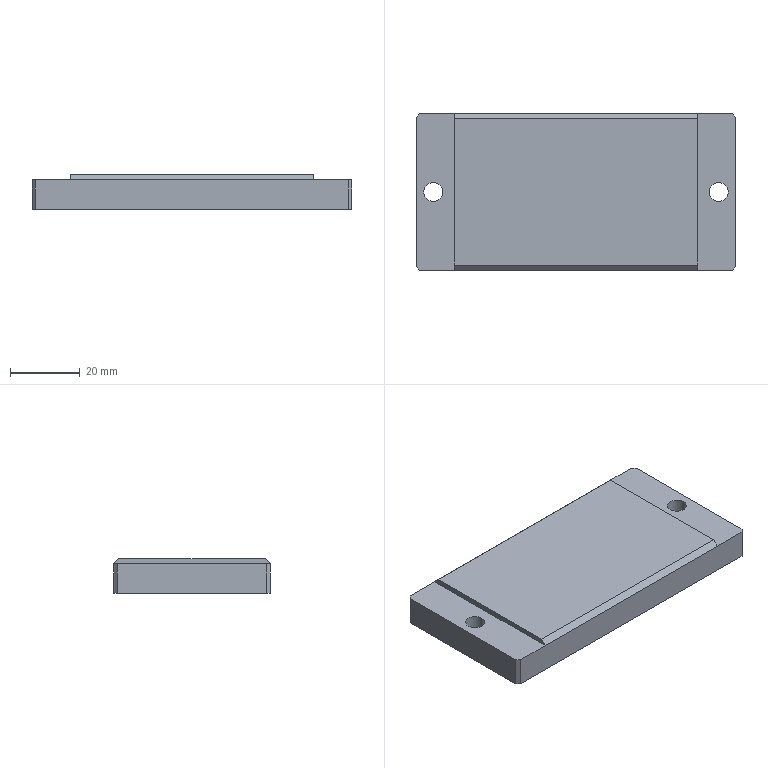Part | STEP file | 2022 Hold-down plate | 1 solid | 20 faces | box 92 x 45 x 10 mm | volume 39337 mm3 | plane 16 | cylinder 4 | commonest cylinder face diameters 5.5 x4
STEP:
#1=CARTESIAN_POINT('',(0.,0.,0.));
#2=DIRECTION('',(0.,0.,1.));
#3=DIRECTION('',(1.,0.,0.));
#4=AXIS2_PLACEMENT_3D('',#1,#2,#3);
#5=CARTESIAN_POINT('',(38.25,0.,8.5));
#6=VERTEX_POINT('',#5);
#7=CARTESIAN_POINT('',(38.25,0.,0.));
#8=VERTEX_POINT('',#7);
#9=CARTESIAN_POINT('',(38.25,0.,10.));
#10=DIRECTION('',(0.,0.,-1.));
#11=VECTOR('',#10,1.);
#12=LINE('',#9,#11);
#13=CARTESIAN_POINT('',(41.,0.,10.));
#14=DIRECTION('',(0.,0.,-1.));
#15=DIRECTION('',(-1.,0.,0.));
#16=AXIS2_PLACEMENT_3D('',#13,#14,#15);
#17=CYLINDRICAL_SURFACE('',#16,2.75);
#18=CARTESIAN_POINT('',(6.283,0.));
#19=DIRECTION('',(0.,1.));
#20=VECTOR('',#19,1.);
#21=LINE('',#18,#20);
#22=(GEOMETRIC_REPRESENTATION_CONTEXT(2)PARAMETRIC_REPRESENTATION_CONTEXT()REPRESENTATION_CONTEXT('',''));
#23=DEFINITIONAL_REPRESENTATION('',(#21),#22);
#24=PCURVE('',#17,#23);
#25=CARTESIAN_POINT('',(41.,0.,10.));
#26=DIRECTION('',(0.,0.,-1.));
#27=DIRECTION('',(-1.,0.,0.));
#28=AXIS2_PLACEMENT_3D('',#25,#26,#27);
#29=CYLINDRICAL_SURFACE('',#28,2.75);
#30=CARTESIAN_POINT('',(0.,0.));
#31=DIRECTION('',(0.,1.));
#32=VECTOR('',#31,1.);
#33=LINE('',#30,#32);
#34=(GEOMETRIC_REPRESENTATION_CONTEXT(2)PARAMETRIC_REPRESENTATION_CONTEXT()REPRESENTATION_CONTEXT('',''));
#35=DEFINITIONAL_REPRESENTATION('',(#33),#34);
#36=PCURVE('',#29,#35);
#37=SURFACE_CURVE('',#12,(#24,#36),.PCURVE_S1.);
#38=EDGE_CURVE('',#6,#8,#37,.T.);
#39=ORIENTED_EDGE('',*,*,#38,.T.);
#40=CARTESIAN_POINT('',(43.75,0.,0.));
#41=VERTEX_POINT('',#40);
#42=CARTESIAN_POINT('',(41.,0.,0.));
#43=DIRECTION('',(0.,0.,-1.));
#44=DIRECTION('',(-1.,0.,0.));
#45=AXIS2_PLACEMENT_3D('',#42,#43,#44);
#46=CIRCLE('',#45,2.75);
#47=CARTESIAN_POINT('',(0.,10.));
#48=DIRECTION('',(1.,0.));
#49=VECTOR('',#48,1.);
#50=LINE('',#47,#49);
#51=(GEOMETRIC_REPRESENTATION_CONTEXT(2)PARAMETRIC_REPRESENTATION_CONTEXT()REPRESENTATION_CONTEXT('',''));
#52=DEFINITIONAL_REPRESENTATION('',(#50),#51);
#53=PCURVE('',#17,#52);
#54=CARTESIAN_POINT('',(0.,0.,0.));
#55=DIRECTION('',(0.,0.,-1.));
#56=DIRECTION('',(-1.,0.,0.));
#57=AXIS2_PLACEMENT_3D('',#54,#55,#56);
#58=PLANE('',#57);
#59=CARTESIAN_POINT('',(-41.,0.));
#60=DIRECTION('',(1.,0.));
#61=AXIS2_PLACEMENT_2D('',#59,#60);
#62=CIRCLE('',#61,2.75);
#63=(GEOMETRIC_REPRESENTATION_CONTEXT(2)PARAMETRIC_REPRESENTATION_CONTEXT()REPRESENTATION_CONTEXT('',''));
#64=DEFINITIONAL_REPRESENTATION('',(#62),#63);
#65=PCURVE('',#58,#64);
#66=SURFACE_CURVE('',#46,(#53,#65),.PCURVE_S1.);
#67=EDGE_CURVE('',#41,#8,#66,.T.);
#68=ORIENTED_EDGE('',*,*,#67,.F.);
#69=CARTESIAN_POINT('',(43.75,0.,8.5));
#70=VERTEX_POINT('',#69);
#71=CARTESIAN_POINT('',(43.75,0.,10.));
#72=DIRECTION('',(0.,0.,-1.));
#73=VECTOR('',#72,1.);
#74=LINE('',#71,#73);
#75=CARTESIAN_POINT('',(3.142,0.));
#76=DIRECTION('',(0.,1.));
#77=VECTOR('',#76,1.);
#78=LINE('',#75,#77);
#79=(GEOMETRIC_REPRESENTATION_CONTEXT(2)PARAMETRIC_REPRESENTATION_CONTEXT()REPRESENTATION_CONTEXT('',''));
#80=DEFINITIONAL_REPRESENTATION('',(#78),#79);
#81=PCURVE('',#17,#80);
#82=CARTESIAN_POINT('',(3.142,0.));
#83=DIRECTION('',(0.,1.));
#84=VECTOR('',#83,1.);
#85=LINE('',#82,#84);
#86=(GEOMETRIC_REPRESENTATION_CONTEXT(2)PARAMETRIC_REPRESENTATION_CONTEXT()REPRESENTATION_CONTEXT('',''));
#87=DEFINITIONAL_REPRESENTATION('',(#85),#86);
#88=PCURVE('',#29,#87);
#89=SURFACE_CURVE('',#74,(#81,#88),.PCURVE_S1.);
#90=EDGE_CURVE('',#70,#41,#89,.T.);
#91=ORIENTED_EDGE('',*,*,#90,.F.);
#92=CARTESIAN_POINT('',(41.,0.,8.5));
#93=DIRECTION('',(0.,0.,-1.));
#94=DIRECTION('',(-1.,0.,0.));
#95=AXIS2_PLACEMENT_3D('',#92,#93,#94);
#96=CIRCLE('',#95,2.75);
#97=CARTESIAN_POINT('',(0.,1.5));
#98=DIRECTION('',(1.,0.));
#99=VECTOR('',#98,1.);
#100=LINE('',#97,#99);
#101=(GEOMETRIC_REPRESENTATION_CONTEXT(2)PARAMETRIC_REPRESENTATION_CONTEXT()REPRESENTATION_CONTEXT('',''));
#102=DEFINITIONAL_REPRESENTATION('',(#100),#101);
#103=PCURVE('',#17,#102);
#104=CARTESIAN_POINT('',(0.,0.,8.5));
#105=DIRECTION('',(0.,0.,-1.));
#106=DIRECTION('',(-1.,0.,0.));
#107=AXIS2_PLACEMENT_3D('',#104,#105,#106);
#108=PLANE('',#107);
#109=CARTESIAN_POINT('',(-41.,0.));
#110=DIRECTION('',(1.,0.));
#111=AXIS2_PLACEMENT_2D('',#109,#110);
#112=CIRCLE('',#111,2.75);
#113=(GEOMETRIC_REPRESENTATION_CONTEXT(2)PARAMETRIC_REPRESENTATION_CONTEXT()REPRESENTATION_CONTEXT('',''));
#114=DEFINITIONAL_REPRESENTATION('',(#112),#113);
#115=PCURVE('',#108,#114);
#116=SURFACE_CURVE('',#96,(#103,#115),.PCURVE_S1.);
#117=EDGE_CURVE('',#70,#6,#116,.T.);
#118=ORIENTED_EDGE('',*,*,#117,.T.);
#119=EDGE_LOOP('',(#39,#68,#91,#118));
#120=FACE_BOUND('',#119,.F.);
#121=ADVANCED_FACE('',(#120),#17,.F.);
#122=CARTESIAN_POINT('',(-43.75,0.,8.5));
#123=VERTEX_POINT('',#122);
#124=CARTESIAN_POINT('',(-43.75,0.,0.));
#125=VERTEX_POINT('',#124);
#126=CARTESIAN_POINT('',(-43.75,0.,10.));
#127=DIRECTION('',(0.,0.,-1.));
#128=VECTOR('',#127,1.);
#129=LINE('',#126,#128);
#130=CARTESIAN_POINT('',(-41.,0.,10.));
#131=DIRECTION('',(0.,0.,-1.));
#132=DIRECTION('',(-1.,0.,0.));
#133=AXIS2_PLACEMENT_3D('',#130,#131,#132);
#134=CYLINDRICAL_SURFACE('',#133,2.75);
#135=CARTESIAN_POINT('',(6.283,0.));
#136=DIRECTION('',(0.,1.));
#137=VECTOR('',#136,1.);
#138=LINE('',#135,#137);
#139=(GEOMETRIC_REPRESENTATION_CONTEXT(2)PARAMETRIC_REPRESENTATION_CONTEXT()REPRESENTATION_CONTEXT('',''));
#140=DEFINITIONAL_REPRESENTATION('',(#138),#139);
#141=PCURVE('',#134,#140);
#142=CARTESIAN_POINT('',(-41.,0.,10.));
#143=DIRECTION('',(0.,0.,-1.));
#144=DIRECTION('',(-1.,0.,0.));
#145=AXIS2_PLACEMENT_3D('',#142,#143,#144);
#146=CYLINDRICAL_SURFACE('',#145,2.75);
#147=CARTESIAN_POINT('',(0.,0.));
#148=DIRECTION('',(0.,1.));
#149=VECTOR('',#148,1.);
#150=LINE('',#147,#149);
#151=(GEOMETRIC_REPRESENTATION_CONTEXT(2)PARAMETRIC_REPRESENTATION_CONTEXT()REPRESENTATION_CONTEXT('',''));
#152=DEFINITIONAL_REPRESENTATION('',(#150),#151);
#153=PCURVE('',#146,#152);
#154=SURFACE_CURVE('',#129,(#141,#153),.PCURVE_S1.);
#155=EDGE_CURVE('',#123,#125,#154,.T.);
#156=ORIENTED_EDGE('',*,*,#155,.T.);
#157=CARTESIAN_POINT('',(-38.25,0.,0.));
#158=VERTEX_POINT('',#157);
#159=CARTESIAN_POINT('',(-41.,0.,0.));
#160=DIRECTION('',(0.,0.,-1.));
#161=DIRECTION('',(-1.,0.,0.));
#162=AXIS2_PLACEMENT_3D('',#159,#160,#161);
#163=CIRCLE('',#162,2.75);
#164=CARTESIAN_POINT('',(0.,10.));
#165=DIRECTION('',(1.,0.));
#166=VECTOR('',#165,1.);
#167=LINE('',#164,#166);
#168=(GEOMETRIC_REPRESENTATION_CONTEXT(2)PARAMETRIC_REPRESENTATION_CONTEXT()REPRESENTATION_CONTEXT('',''));
#169=DEFINITIONAL_REPRESENTATION('',(#167),#168);
#170=PCURVE('',#134,#169);
#171=CARTESIAN_POINT('',(41.,0.));
#172=DIRECTION('',(1.,0.));
#173=AXIS2_PLACEMENT_2D('',#171,#172);
#174=CIRCLE('',#173,2.75);
#175=(GEOMETRIC_REPRESENTATION_CONTEXT(2)PARAMETRIC_REPRESENTATION_CONTEXT()REPRESENTATION_CONTEXT('',''));
#176=DEFINITIONAL_REPRESENTATION('',(#174),#175);
#177=PCURVE('',#58,#176);
#178=SURFACE_CURVE('',#163,(#170,#177),.PCURVE_S1.);
#179=EDGE_CURVE('',#158,#125,#178,.T.);
#180=ORIENTED_EDGE('',*,*,#179,.F.);
#181=CARTESIAN_POINT('',(-38.25,0.,8.5));
#182=VERTEX_POINT('',#181);
#183=CARTESIAN_POINT('',(-38.25,0.,10.));
#184=DIRECTION('',(0.,0.,-1.));
#185=VECTOR('',#184,1.);
#186=LINE('',#183,#185);
#187=CARTESIAN_POINT('',(3.142,0.));
#188=DIRECTION('',(0.,1.));
#189=VECTOR('',#188,1.);
#190=LINE('',#187,#189);
#191=(GEOMETRIC_REPRESENTATION_CONTEXT(2)PARAMETRIC_REPRESENTATION_CONTEXT()REPRESENTATION_CONTEXT('',''));
#192=DEFINITIONAL_REPRESENTATION('',(#190),#191);
#193=PCURVE('',#134,#192);
#194=CARTESIAN_POINT('',(3.142,0.));
#195=DIRECTION('',(0.,1.));
#196=VECTOR('',#195,1.);
#197=LINE('',#194,#196);
#198=(GEOMETRIC_REPRESENTATION_CONTEXT(2)PARAMETRIC_REPRESENTATION_CONTEXT()REPRESENTATION_CONTEXT('',''));
#199=DEFINITIONAL_REPRESENTATION('',(#197),#198);
#200=PCURVE('',#146,#199);
#201=SURFACE_CURVE('',#186,(#193,#200),.PCURVE_S1.);
#202=EDGE_CURVE('',#182,#158,#201,.T.);
#203=ORIENTED_EDGE('',*,*,#202,.F.);
#204=CARTESIAN_POINT('',(-41.,0.,8.5));
#205=DIRECTION('',(0.,0.,1.));
#206=DIRECTION('',(1.,0.,0.));
#207=AXIS2_PLACEMENT_3D('',#204,#205,#206);
#208=CIRCLE('',#207,2.75);
#209=CARTESIAN_POINT('',(9.425,1.5));
#210=DIRECTION('',(-1.,0.));
#211=VECTOR('',#210,1.);
#212=LINE('',#209,#211);
#213=(GEOMETRIC_REPRESENTATION_CONTEXT(2)PARAMETRIC_REPRESENTATION_CONTEXT()REPRESENTATION_CONTEXT('',''));
#214=DEFINITIONAL_REPRESENTATION('',(#212),#213);
#215=PCURVE('',#134,#214);
#216=CARTESIAN_POINT('',(0.,0.,8.5));
#217=DIRECTION('',(0.,0.,1.));
#218=DIRECTION('',(1.,0.,0.));
#219=AXIS2_PLACEMENT_3D('',#216,#217,#218);
#220=PLANE('',#219);
#221=CARTESIAN_POINT('',(-41.,0.));
#222=DIRECTION('',(1.,0.));
#223=AXIS2_PLACEMENT_2D('',#221,#222);
#224=CIRCLE('',#223,2.75);
#225=(GEOMETRIC_REPRESENTATION_CONTEXT(2)PARAMETRIC_REPRESENTATION_CONTEXT()REPRESENTATION_CONTEXT('',''));
#226=DEFINITIONAL_REPRESENTATION('',(#224),#225);
#227=PCURVE('',#220,#226);
#228=SURFACE_CURVE('',#208,(#215,#227),.PCURVE_S1.);
#229=EDGE_CURVE('',#123,#182,#228,.T.);
#230=ORIENTED_EDGE('',*,*,#229,.F.);
#231=EDGE_LOOP('',(#156,#180,#203,#230));
#232=FACE_BOUND('',#231,.F.);
#233=ADVANCED_FACE('',(#232),#134,.F.);
#234=CARTESIAN_POINT('',(-46.,21.5,0.));
#235=VERTEX_POINT('',#234);
#236=CARTESIAN_POINT('',(-46.,-21.5,0.));
#237=VERTEX_POINT('',#236);
#238=CARTESIAN_POINT('',(-46.,-22.5,0.));
#239=DIRECTION('',(0.,-1.,0.));
#240=VECTOR('',#239,1.);
#241=LINE('',#238,#240);
#242=CARTESIAN_POINT('',(-46.,-22.5,10.));
#243=DIRECTION('',(1.,0.,0.));
#244=DIRECTION('',(0.,0.,-1.));
#245=AXIS2_PLACEMENT_3D('',#242,#243,#244);
#246=PLANE('',#245);
#247=CARTESIAN_POINT('',(10.,0.));
#248=DIRECTION('',(0.,-1.));
#249=VECTOR('',#248,1.);
#250=LINE('',#247,#249);
#251=(GEOMETRIC_REPRESENTATION_CONTEXT(2)PARAMETRIC_REPRESENTATION_CONTEXT()REPRESENTATION_CONTEXT('',''));
#252=DEFINITIONAL_REPRESENTATION('',(#250),#251);
#253=PCURVE('',#246,#252);
#254=CARTESIAN_POINT('',(46.,-22.5));
#255=DIRECTION('',(0.,-1.));
#256=VECTOR('',#255,1.);
#257=LINE('',#254,#256);
#258=(GEOMETRIC_REPRESENTATION_CONTEXT(2)PARAMETRIC_REPRESENTATION_CONTEXT()REPRESENTATION_CONTEXT('',''));
#259=DEFINITIONAL_REPRESENTATION('',(#257),#258);
#260=PCURVE('',#58,#259);
#261=SURFACE_CURVE('',#241,(#253,#260),.PCURVE_S1.);
#262=EDGE_CURVE('',#235,#237,#261,.T.);
#263=ORIENTED_EDGE('',*,*,#262,.T.);
#264=CARTESIAN_POINT('',(-46.,-21.5,8.5));
#265=VERTEX_POINT('',#264);
#266=CARTESIAN_POINT('',(-46.,-21.5,10.));
#267=DIRECTION('',(0.,0.,1.));
#268=VECTOR('',#267,1.);
#269=LINE('',#266,#268);
#270=CARTESIAN_POINT('',(0.,1.));
#271=DIRECTION('',(-1.,0.));
#272=VECTOR('',#271,1.);
#273=LINE('',#270,#272);
#274=(GEOMETRIC_REPRESENTATION_CONTEXT(2)PARAMETRIC_REPRESENTATION_CONTEXT()REPRESENTATION_CONTEXT('',''));
#275=DEFINITIONAL_REPRESENTATION('',(#273),#274);
#276=PCURVE('',#246,#275);
#277=CARTESIAN_POINT('',(-45.,-22.5,10.));
#278=DIRECTION('',(0.7071,0.7071,0.));
#279=DIRECTION('',(0.,0.,-1.));
#280=AXIS2_PLACEMENT_3D('',#277,#278,#279);
#281=PLANE('',#280);
#282=CARTESIAN_POINT('',(0.,1.414));
#283=DIRECTION('',(-1.,0.));
#284=VECTOR('',#283,1.);
#285=LINE('',#282,#284);
#286=(GEOMETRIC_REPRESENTATION_CONTEXT(2)PARAMETRIC_REPRESENTATION_CONTEXT()REPRESENTATION_CONTEXT('',''));
#287=DEFINITIONAL_REPRESENTATION('',(#285),#286);
#288=PCURVE('',#281,#287);
#289=SURFACE_CURVE('',#269,(#276,#288),.PCURVE_S1.);
#290=EDGE_CURVE('',#237,#265,#289,.T.);
#291=ORIENTED_EDGE('',*,*,#290,.T.);
#292=CARTESIAN_POINT('',(-46.,21.5,8.5));
#293=VERTEX_POINT('',#292);
#294=CARTESIAN_POINT('',(-46.,22.5,8.5));
#295=DIRECTION('',(0.,-1.,0.));
#296=VECTOR('',#295,1.);
#297=LINE('',#294,#296);
#298=CARTESIAN_POINT('',(1.5,45.));
#299=DIRECTION('',(0.,-1.));
#300=VECTOR('',#299,1.);
#301=LINE('',#298,#300);
#302=(GEOMETRIC_REPRESENTATION_CONTEXT(2)PARAMETRIC_REPRESENTATION_CONTEXT()REPRESENTATION_CONTEXT('',''));
#303=DEFINITIONAL_REPRESENTATION('',(#301),#302);
#304=PCURVE('',#246,#303);
#305=CARTESIAN_POINT('',(-46.,22.5));
#306=DIRECTION('',(0.,-1.));
#307=VECTOR('',#306,1.);
#308=LINE('',#305,#307);
#309=(GEOMETRIC_REPRESENTATION_CONTEXT(2)PARAMETRIC_REPRESENTATION_CONTEXT()REPRESENTATION_CONTEXT('',''));
#310=DEFINITIONAL_REPRESENTATION('',(#308),#309);
#311=PCURVE('',#220,#310);
#312=SURFACE_CURVE('',#297,(#304,#311),.PCURVE_S1.);
#313=EDGE_CURVE('',#293,#265,#312,.T.);
#314=ORIENTED_EDGE('',*,*,#313,.F.);
#315=CARTESIAN_POINT('',(-46.,21.5,10.));
#316=DIRECTION('',(0.,0.,-1.));
#317=VECTOR('',#316,1.);
#318=LINE('',#315,#317);
#319=CARTESIAN_POINT('',(0.,44.));
#320=DIRECTION('',(1.,0.));
#321=VECTOR('',#320,1.);
#322=LINE('',#319,#321);
#323=(GEOMETRIC_REPRESENTATION_CONTEXT(2)PARAMETRIC_REPRESENTATION_CONTEXT()REPRESENTATION_CONTEXT('',''));
#324=DEFINITIONAL_REPRESENTATION('',(#322),#323);
#325=PCURVE('',#246,#324);
#326=CARTESIAN_POINT('',(-46.,21.5,10.));
#327=DIRECTION('',(0.7071,-0.7071,0.));
#328=DIRECTION('',(0.,0.,-1.));
#329=AXIS2_PLACEMENT_3D('',#326,#327,#328);
#330=PLANE('',#329);
#331=CARTESIAN_POINT('',(0.,0.));
#332=DIRECTION('',(1.,0.));
#333=VECTOR('',#332,1.);
#334=LINE('',#331,#333);
#335=(GEOMETRIC_REPRESENTATION_CONTEXT(2)PARAMETRIC_REPRESENTATION_CONTEXT()REPRESENTATION_CONTEXT('',''));
#336=DEFINITIONAL_REPRESENTATION('',(#334),#335);
#337=PCURVE('',#330,#336);
#338=SURFACE_CURVE('',#318,(#325,#337),.PCURVE_S1.);
#339=EDGE_CURVE('',#293,#235,#338,.T.);
#340=ORIENTED_EDGE('',*,*,#339,.T.);
#341=EDGE_LOOP('',(#263,#291,#314,#340));
#342=FACE_BOUND('',#341,.T.);
#343=ADVANCED_FACE('',(#342),#246,.F.);
#344=CARTESIAN_POINT('',(46.,-21.5,8.5));
#345=VERTEX_POINT('',#344);
#346=CARTESIAN_POINT('',(46.,21.5,8.5));
#347=VERTEX_POINT('',#346);
#348=CARTESIAN_POINT('',(46.,22.5,8.5));
#349=DIRECTION('',(0.,1.,0.));
#350=VECTOR('',#349,1.);
#351=LINE('',#348,#350);
#352=CARTESIAN_POINT('',(46.,-22.5,10.));
#353=DIRECTION('',(-1.,0.,0.));
#354=DIRECTION('',(0.,0.,1.));
#355=AXIS2_PLACEMENT_3D('',#352,#353,#354);
#356=PLANE('',#355);
#357=CARTESIAN_POINT('',(-1.5,45.));
#358=DIRECTION('',(0.,1.));
#359=VECTOR('',#358,1.);
#360=LINE('',#357,#359);
#361=(GEOMETRIC_REPRESENTATION_CONTEXT(2)PARAMETRIC_REPRESENTATION_CONTEXT()REPRESENTATION_CONTEXT('',''));
#362=DEFINITIONAL_REPRESENTATION('',(#360),#361);
#363=PCURVE('',#356,#362);
#364=CARTESIAN_POINT('',(-46.,22.5));
#365=DIRECTION('',(0.,1.));
#366=VECTOR('',#365,1.);
#367=LINE('',#364,#366);
#368=(GEOMETRIC_REPRESENTATION_CONTEXT(2)PARAMETRIC_REPRESENTATION_CONTEXT()REPRESENTATION_CONTEXT('',''));
#369=DEFINITIONAL_REPRESENTATION('',(#367),#368);
#370=PCURVE('',#108,#369);
#371=SURFACE_CURVE('',#351,(#363,#370),.PCURVE_S1.);
#372=EDGE_CURVE('',#345,#347,#371,.T.);
#373=ORIENTED_EDGE('',*,*,#372,.F.);
#374=CARTESIAN_POINT('',(46.,-21.5,0.));
#375=VERTEX_POINT('',#374);
#376=CARTESIAN_POINT('',(46.,-21.5,10.));
#377=DIRECTION('',(0.,0.,-1.));
#378=VECTOR('',#377,1.);
#379=LINE('',#376,#378);
#380=CARTESIAN_POINT('',(0.,1.));
#381=DIRECTION('',(-1.,0.));
#382=VECTOR('',#381,1.);
#383=LINE('',#380,#382);
#384=(GEOMETRIC_REPRESENTATION_CONTEXT(2)PARAMETRIC_REPRESENTATION_CONTEXT()REPRESENTATION_CONTEXT('',''));
#385=DEFINITIONAL_REPRESENTATION('',(#383),#384);
#386=PCURVE('',#356,#385);
#387=CARTESIAN_POINT('',(46.,-21.5,10.));
#388=DIRECTION('',(-0.7071,0.7071,0.));
#389=DIRECTION('',(0.,0.,-1.));
#390=AXIS2_PLACEMENT_3D('',#387,#388,#389);
#391=PLANE('',#390);
#392=CARTESIAN_POINT('',(0.,0.));
#393=DIRECTION('',(1.,0.));
#394=VECTOR('',#393,1.);
#395=LINE('',#392,#394);
#396=(GEOMETRIC_REPRESENTATION_CONTEXT(2)PARAMETRIC_REPRESENTATION_CONTEXT()REPRESENTATION_CONTEXT('',''));
#397=DEFINITIONAL_REPRESENTATION('',(#395),#396);
#398=PCURVE('',#391,#397);
#399=SURFACE_CURVE('',#379,(#386,#398),.PCURVE_S1.);
#400=EDGE_CURVE('',#345,#375,#399,.T.);
#401=ORIENTED_EDGE('',*,*,#400,.T.);
#402=CARTESIAN_POINT('',(46.,21.5,0.));
#403=VERTEX_POINT('',#402);
#404=CARTESIAN_POINT('',(46.,-22.5,0.));
#405=DIRECTION('',(0.,1.,0.));
#406=VECTOR('',#405,1.);
#407=LINE('',#404,#406);
#408=CARTESIAN_POINT('',(-10.,0.));
#409=DIRECTION('',(0.,1.));
#410=VECTOR('',#409,1.);
#411=LINE('',#408,#410);
#412=(GEOMETRIC_REPRESENTATION_CONTEXT(2)PARAMETRIC_REPRESENTATION_CONTEXT()REPRESENTATION_CONTEXT('',''));
#413=DEFINITIONAL_REPRESENTATION('',(#411),#412);
#414=PCURVE('',#356,#413);
#415=CARTESIAN_POINT('',(-46.,-22.5));
#416=DIRECTION('',(0.,1.));
#417=VECTOR('',#416,1.);
#418=LINE('',#415,#417);
#419=(GEOMETRIC_REPRESENTATION_CONTEXT(2)PARAMETRIC_REPRESENTATION_CONTEXT()REPRESENTATION_CONTEXT('',''));
#420=DEFINITIONAL_REPRESENTATION('',(#418),#419);
#421=PCURVE('',#58,#420);
#422=SURFACE_CURVE('',#407,(#414,#421),.PCURVE_S1.);
#423=EDGE_CURVE('',#375,#403,#422,.T.);
#424=ORIENTED_EDGE('',*,*,#423,.T.);
#425=CARTESIAN_POINT('',(46.,21.5,10.));
#426=DIRECTION('',(0.,0.,1.));
#427=VECTOR('',#426,1.);
#428=LINE('',#425,#427);
#429=CARTESIAN_POINT('',(0.,44.));
#430=DIRECTION('',(1.,0.));
#431=VECTOR('',#430,1.);
#432=LINE('',#429,#431);
#433=(GEOMETRIC_REPRESENTATION_CONTEXT(2)PARAMETRIC_REPRESENTATION_CONTEXT()REPRESENTATION_CONTEXT('',''));
#434=DEFINITIONAL_REPRESENTATION('',(#432),#433);
#435=PCURVE('',#356,#434);
#436=CARTESIAN_POINT('',(45.,22.5,10.));
#437=DIRECTION('',(-0.7071,-0.7071,0.));
#438=DIRECTION('',(0.,0.,-1.));
#439=AXIS2_PLACEMENT_3D('',#436,#437,#438);
#440=PLANE('',#439);
#441=CARTESIAN_POINT('',(0.,1.414));
#442=DIRECTION('',(-1.,0.));
#443=VECTOR('',#442,1.);
#444=LINE('',#441,#443);
#445=(GEOMETRIC_REPRESENTATION_CONTEXT(2)PARAMETRIC_REPRESENTATION_CONTEXT()REPRESENTATION_CONTEXT('',''));
#446=DEFINITIONAL_REPRESENTATION('',(#444),#445);
#447=PCURVE('',#440,#446);
#448=SURFACE_CURVE('',#428,(#435,#447),.PCURVE_S1.);
#449=EDGE_CURVE('',#403,#347,#448,.T.);
#450=ORIENTED_EDGE('',*,*,#449,.T.);
#451=EDGE_LOOP('',(#373,#401,#424,#450));
#452=FACE_BOUND('',#451,.T.);
#453=ADVANCED_FACE('',(#452),#356,.F.);
#454=CARTESIAN_POINT('',(-35.,22.5,8.5));
#455=VERTEX_POINT('',#454);
#456=CARTESIAN_POINT('',(-45.,22.5,8.5));
#457=VERTEX_POINT('',#456);
#458=CARTESIAN_POINT('',(-46.,22.5,8.5));
#459=DIRECTION('',(-1.,0.,0.));
#460=VECTOR('',#459,1.);
#461=LINE('',#458,#460);
#462=CARTESIAN_POINT('',(-46.,22.5,10.));
#463=DIRECTION('',(0.,-1.,0.));
#464=DIRECTION('',(0.,0.,-1.));
#465=AXIS2_PLACEMENT_3D('',#462,#463,#464);
#466=PLANE('',#465);
#467=CARTESIAN_POINT('',(1.5,0.));
#468=DIRECTION('',(0.,-1.));
#469=VECTOR('',#468,1.);
#470=LINE('',#467,#469);
#471=(GEOMETRIC_REPRESENTATION_CONTEXT(2)PARAMETRIC_REPRESENTATION_CONTEXT()REPRESENTATION_CONTEXT('',''));
#472=DEFINITIONAL_REPRESENTATION('',(#470),#471);
#473=PCURVE('',#466,#472);
#474=CARTESIAN_POINT('',(-46.,22.5));
#475=DIRECTION('',(-1.,0.));
#476=VECTOR('',#475,1.);
#477=LINE('',#474,#476);
#478=(GEOMETRIC_REPRESENTATION_CONTEXT(2)PARAMETRIC_REPRESENTATION_CONTEXT()REPRESENTATION_CONTEXT('',''));
#479=DEFINITIONAL_REPRESENTATION('',(#477),#478);
#480=PCURVE('',#220,#479);
#481=SURFACE_CURVE('',#461,(#473,#480),.PCURVE_S1.);
#482=EDGE_CURVE('',#455,#457,#481,.T.);
#483=ORIENTED_EDGE('',*,*,#482,.F.);
#484=CARTESIAN_POINT('',(35.,22.5,8.5));
#485=VERTEX_POINT('',#484);
#486=CARTESIAN_POINT('',(-46.,22.5,8.5));
#487=DIRECTION('',(1.,0.,0.));
#488=VECTOR('',#487,1.);
#489=LINE('',#486,#488);
#490=CARTESIAN_POINT('',(1.5,0.));
#491=DIRECTION('',(0.,1.));
#492=VECTOR('',#491,1.);
#493=LINE('',#490,#492);
#494=(GEOMETRIC_REPRESENTATION_CONTEXT(2)PARAMETRIC_REPRESENTATION_CONTEXT()REPRESENTATION_CONTEXT('',''));
#495=DEFINITIONAL_REPRESENTATION('',(#493),#494);
#496=PCURVE('',#466,#495);
#497=CARTESIAN_POINT('',(0.,21.,10.));
#498=DIRECTION('',(0.,-0.7071,-0.7071));
#499=DIRECTION('',(-1.,0.,0.));
#500=AXIS2_PLACEMENT_3D('',#497,#498,#499);
#501=PLANE('',#500);
#502=CARTESIAN_POINT('',(46.,2.121));
#503=DIRECTION('',(-1.,0.));
#504=VECTOR('',#503,1.);
#505=LINE('',#502,#504);
#506=(GEOMETRIC_REPRESENTATION_CONTEXT(2)PARAMETRIC_REPRESENTATION_CONTEXT()REPRESENTATION_CONTEXT('',''));
#507=DEFINITIONAL_REPRESENTATION('',(#505),#506);
#508=PCURVE('',#501,#507);
#509=SURFACE_CURVE('',#489,(#496,#508),.PCURVE_S1.);
#510=EDGE_CURVE('',#455,#485,#509,.T.);
#511=ORIENTED_EDGE('',*,*,#510,.T.);
#512=CARTESIAN_POINT('',(45.,22.5,8.5));
#513=VERTEX_POINT('',#512);
#514=CARTESIAN_POINT('',(46.,22.5,8.5));
#515=DIRECTION('',(-1.,0.,0.));
#516=VECTOR('',#515,1.);
#517=LINE('',#514,#516);
#518=CARTESIAN_POINT('',(1.5,92.));
#519=DIRECTION('',(0.,-1.));
#520=VECTOR('',#519,1.);
#521=LINE('',#518,#520);
#522=(GEOMETRIC_REPRESENTATION_CONTEXT(2)PARAMETRIC_REPRESENTATION_CONTEXT()REPRESENTATION_CONTEXT('',''));
#523=DEFINITIONAL_REPRESENTATION('',(#521),#522);
#524=PCURVE('',#466,#523);
#525=CARTESIAN_POINT('',(-46.,22.5));
#526=DIRECTION('',(1.,0.));
#527=VECTOR('',#526,1.);
#528=LINE('',#525,#527);
#529=(GEOMETRIC_REPRESENTATION_CONTEXT(2)PARAMETRIC_REPRESENTATION_CONTEXT()REPRESENTATION_CONTEXT('',''));
#530=DEFINITIONAL_REPRESENTATION('',(#528),#529);
#531=PCURVE('',#108,#530);
#532=SURFACE_CURVE('',#517,(#524,#531),.PCURVE_S1.);
#533=EDGE_CURVE('',#513,#485,#532,.T.);
#534=ORIENTED_EDGE('',*,*,#533,.F.);
#535=CARTESIAN_POINT('',(45.,22.5,0.));
#536=VERTEX_POINT('',#535);
#537=CARTESIAN_POINT('',(45.,22.5,10.));
#538=DIRECTION('',(0.,0.,-1.));
#539=VECTOR('',#538,1.);
#540=LINE('',#537,#539);
#541=CARTESIAN_POINT('',(0.,91.));
#542=DIRECTION('',(1.,0.));
#543=VECTOR('',#542,1.);
#544=LINE('',#541,#543);
#545=(GEOMETRIC_REPRESENTATION_CONTEXT(2)PARAMETRIC_REPRESENTATION_CONTEXT()REPRESENTATION_CONTEXT('',''));
#546=DEFINITIONAL_REPRESENTATION('',(#544),#545);
#547=PCURVE('',#466,#546);
#548=CARTESIAN_POINT('',(0.,0.));
#549=DIRECTION('',(1.,0.));
#550=VECTOR('',#549,1.);
#551=LINE('',#548,#550);
#552=(GEOMETRIC_REPRESENTATION_CONTEXT(2)PARAMETRIC_REPRESENTATION_CONTEXT()REPRESENTATION_CONTEXT('',''));
#553=DEFINITIONAL_REPRESENTATION('',(#551),#552);
#554=PCURVE('',#440,#553);
#555=SURFACE_CURVE('',#540,(#547,#554),.PCURVE_S1.);
#556=EDGE_CURVE('',#513,#536,#555,.T.);
#557=ORIENTED_EDGE('',*,*,#556,.T.);
#558=CARTESIAN_POINT('',(-45.,22.5,0.));
#559=VERTEX_POINT('',#558);
#560=CARTESIAN_POINT('',(-46.,22.5,0.));
#561=DIRECTION('',(-1.,0.,0.));
#562=VECTOR('',#561,1.);
#563=LINE('',#560,#562);
#564=CARTESIAN_POINT('',(10.,0.));
#565=DIRECTION('',(0.,-1.));
#566=VECTOR('',#565,1.);
#567=LINE('',#564,#566);
#568=(GEOMETRIC_REPRESENTATION_CONTEXT(2)PARAMETRIC_REPRESENTATION_CONTEXT()REPRESENTATION_CONTEXT('',''));
#569=DEFINITIONAL_REPRESENTATION('',(#567),#568);
#570=PCURVE('',#466,#569);
#571=CARTESIAN_POINT('',(46.,22.5));
#572=DIRECTION('',(1.,0.));
#573=VECTOR('',#572,1.);
#574=LINE('',#571,#573);
#575=(GEOMETRIC_REPRESENTATION_CONTEXT(2)PARAMETRIC_REPRESENTATION_CONTEXT()REPRESENTATION_CONTEXT('',''));
#576=DEFINITIONAL_REPRESENTATION('',(#574),#575);
#577=PCURVE('',#58,#576);
#578=SURFACE_CURVE('',#563,(#570,#577),.PCURVE_S1.);
#579=EDGE_CURVE('',#536,#559,#578,.T.);
#580=ORIENTED_EDGE('',*,*,#579,.T.);
#581=CARTESIAN_POINT('',(-45.,22.5,10.));
#582=DIRECTION('',(0.,0.,1.));
#583=VECTOR('',#582,1.);
#584=LINE('',#581,#583);
#585=CARTESIAN_POINT('',(0.,1.));
#586=DIRECTION('',(-1.,0.));
#587=VECTOR('',#586,1.);
#588=LINE('',#585,#587);
#589=(GEOMETRIC_REPRESENTATION_CONTEXT(2)PARAMETRIC_REPRESENTATION_CONTEXT()REPRESENTATION_CONTEXT('',''));
#590=DEFINITIONAL_REPRESENTATION('',(#588),#589);
#591=PCURVE('',#466,#590);
#592=CARTESIAN_POINT('',(0.,1.414));
#593=DIRECTION('',(-1.,0.));
#594=VECTOR('',#593,1.);
#595=LINE('',#592,#594);
#596=(GEOMETRIC_REPRESENTATION_CONTEXT(2)PARAMETRIC_REPRESENTATION_CONTEXT()REPRESENTATION_CONTEXT('',''));
#597=DEFINITIONAL_REPRESENTATION('',(#595),#596);
#598=PCURVE('',#330,#597);
#599=SURFACE_CURVE('',#584,(#591,#598),.PCURVE_S1.);
#600=EDGE_CURVE('',#559,#457,#599,.T.);
#601=ORIENTED_EDGE('',*,*,#600,.T.);
#602=EDGE_LOOP('',(#483,#511,#534,#557,#580,#601));
#603=FACE_BOUND('',#602,.T.);
#604=ADVANCED_FACE('',(#603),#466,.F.);
#605=CARTESIAN_POINT('',(35.,-22.5,8.5));
#606=VERTEX_POINT('',#605);
#607=CARTESIAN_POINT('',(45.,-22.5,8.5));
#608=VERTEX_POINT('',#607);
#609=CARTESIAN_POINT('',(46.,-22.5,8.5));
#610=DIRECTION('',(1.,0.,0.));
#611=VECTOR('',#610,1.);
#612=LINE('',#609,#611);
#613=CARTESIAN_POINT('',(-46.,-22.5,10.));
#614=DIRECTION('',(0.,1.,0.));
#615=DIRECTION('',(0.,0.,1.));
#616=AXIS2_PLACEMENT_3D('',#613,#614,#615);
#617=PLANE('',#616);
#618=CARTESIAN_POINT('',(-1.5,92.));
#619=DIRECTION('',(0.,1.));
#620=VECTOR('',#619,1.);
#621=LINE('',#618,#620);
#622=(GEOMETRIC_REPRESENTATION_CONTEXT(2)PARAMETRIC_REPRESENTATION_CONTEXT()REPRESENTATION_CONTEXT('',''));
#623=DEFINITIONAL_REPRESENTATION('',(#621),#622);
#624=PCURVE('',#617,#623);
#625=CARTESIAN_POINT('',(-46.,-22.5));
#626=DIRECTION('',(-1.,0.));
#627=VECTOR('',#626,1.);
#628=LINE('',#625,#627);
#629=(GEOMETRIC_REPRESENTATION_CONTEXT(2)PARAMETRIC_REPRESENTATION_CONTEXT()REPRESENTATION_CONTEXT('',''));
#630=DEFINITIONAL_REPRESENTATION('',(#628),#629);
#631=PCURVE('',#108,#630);
#632=SURFACE_CURVE('',#612,(#624,#631),.PCURVE_S1.);
#633=EDGE_CURVE('',#606,#608,#632,.T.);
#634=ORIENTED_EDGE('',*,*,#633,.F.);
#635=CARTESIAN_POINT('',(-35.,-22.5,8.5));
#636=VERTEX_POINT('',#635);
#637=CARTESIAN_POINT('',(-46.,-22.5,8.5));
#638=DIRECTION('',(-1.,0.,0.));
#639=VECTOR('',#638,1.);
#640=LINE('',#637,#639);
#641=CARTESIAN_POINT('',(-1.5,0.));
#642=DIRECTION('',(0.,-1.));
#643=VECTOR('',#642,1.);
#644=LINE('',#641,#643);
#645=(GEOMETRIC_REPRESENTATION_CONTEXT(2)PARAMETRIC_REPRESENTATION_CONTEXT()REPRESENTATION_CONTEXT('',''));
#646=DEFINITIONAL_REPRESENTATION('',(#644),#645);
#647=PCURVE('',#617,#646);
#648=CARTESIAN_POINT('',(0.,-21.,10.));
#649=DIRECTION('',(0.,0.7071,-0.7071));
#650=DIRECTION('',(1.,0.,0.));
#651=AXIS2_PLACEMENT_3D('',#648,#649,#650);
#652=PLANE('',#651);
#653=CARTESIAN_POINT('',(-46.,2.121));
#654=DIRECTION('',(-1.,0.));
#655=VECTOR('',#654,1.);
#656=LINE('',#653,#655);
#657=(GEOMETRIC_REPRESENTATION_CONTEXT(2)PARAMETRIC_REPRESENTATION_CONTEXT()REPRESENTATION_CONTEXT('',''));
#658=DEFINITIONAL_REPRESENTATION('',(#656),#657);
#659=PCURVE('',#652,#658);
#660=SURFACE_CURVE('',#640,(#647,#659),.PCURVE_S1.);
#661=EDGE_CURVE('',#606,#636,#660,.T.);
#662=ORIENTED_EDGE('',*,*,#661,.T.);
#663=CARTESIAN_POINT('',(-45.,-22.5,8.5));
#664=VERTEX_POINT('',#663);
#665=CARTESIAN_POINT('',(-46.,-22.5,8.5));
#666=DIRECTION('',(1.,0.,0.));
#667=VECTOR('',#666,1.);
#668=LINE('',#665,#667);
#669=CARTESIAN_POINT('',(-1.5,0.));
#670=DIRECTION('',(0.,1.));
#671=VECTOR('',#670,1.);
#672=LINE('',#669,#671);
#673=(GEOMETRIC_REPRESENTATION_CONTEXT(2)PARAMETRIC_REPRESENTATION_CONTEXT()REPRESENTATION_CONTEXT('',''));
#674=DEFINITIONAL_REPRESENTATION('',(#672),#673);
#675=PCURVE('',#617,#674);
#676=CARTESIAN_POINT('',(-46.,-22.5));
#677=DIRECTION('',(1.,0.));
#678=VECTOR('',#677,1.);
#679=LINE('',#676,#678);
#680=(GEOMETRIC_REPRESENTATION_CONTEXT(2)PARAMETRIC_REPRESENTATION_CONTEXT()REPRESENTATION_CONTEXT('',''));
#681=DEFINITIONAL_REPRESENTATION('',(#679),#680);
#682=PCURVE('',#220,#681);
#683=SURFACE_CURVE('',#668,(#675,#682),.PCURVE_S1.);
#684=EDGE_CURVE('',#664,#636,#683,.T.);
#685=ORIENTED_EDGE('',*,*,#684,.F.);
#686=CARTESIAN_POINT('',(-45.,-22.5,0.));
#687=VERTEX_POINT('',#686);
#688=CARTESIAN_POINT('',(-45.,-22.5,10.));
#689=DIRECTION('',(0.,0.,-1.));
#690=VECTOR('',#689,1.);
#691=LINE('',#688,#690);
#692=CARTESIAN_POINT('',(0.,1.));
#693=DIRECTION('',(-1.,0.));
#694=VECTOR('',#693,1.);
#695=LINE('',#692,#694);
#696=(GEOMETRIC_REPRESENTATION_CONTEXT(2)PARAMETRIC_REPRESENTATION_CONTEXT()REPRESENTATION_CONTEXT('',''));
#697=DEFINITIONAL_REPRESENTATION('',(#695),#696);
#698=PCURVE('',#617,#697);
#699=CARTESIAN_POINT('',(0.,0.));
#700=DIRECTION('',(1.,0.));
#701=VECTOR('',#700,1.);
#702=LINE('',#699,#701);
#703=(GEOMETRIC_REPRESENTATION_CONTEXT(2)PARAMETRIC_REPRESENTATION_CONTEXT()REPRESENTATION_CONTEXT('',''));
#704=DEFINITIONAL_REPRESENTATION('',(#702),#703);
#705=PCURVE('',#281,#704);
#706=SURFACE_CURVE('',#691,(#698,#705),.PCURVE_S1.);
#707=EDGE_CURVE('',#664,#687,#706,.T.);
#708=ORIENTED_EDGE('',*,*,#707,.T.);
#709=CARTESIAN_POINT('',(45.,-22.5,0.));
#710=VERTEX_POINT('',#709);
#711=CARTESIAN_POINT('',(-46.,-22.5,0.));
#712=DIRECTION('',(1.,0.,0.));
#713=VECTOR('',#712,1.);
#714=LINE('',#711,#713);
#715=CARTESIAN_POINT('',(-10.,0.));
#716=DIRECTION('',(0.,1.));
#717=VECTOR('',#716,1.);
#718=LINE('',#715,#717);
#719=(GEOMETRIC_REPRESENTATION_CONTEXT(2)PARAMETRIC_REPRESENTATION_CONTEXT()REPRESENTATION_CONTEXT('',''));
#720=DEFINITIONAL_REPRESENTATION('',(#718),#719);
#721=PCURVE('',#617,#720);
#722=CARTESIAN_POINT('',(46.,-22.5));
#723=DIRECTION('',(-1.,0.));
#724=VECTOR('',#723,1.);
#725=LINE('',#722,#724);
#726=(GEOMETRIC_REPRESENTATION_CONTEXT(2)PARAMETRIC_REPRESENTATION_CONTEXT()REPRESENTATION_CONTEXT('',''));
#727=DEFINITIONAL_REPRESENTATION('',(#725),#726);
#728=PCURVE('',#58,#727);
#729=SURFACE_CURVE('',#714,(#721,#728),.PCURVE_S1.);
#730=EDGE_CURVE('',#687,#710,#729,.T.);
#731=ORIENTED_EDGE('',*,*,#730,.T.);
#732=CARTESIAN_POINT('',(45.,-22.5,10.));
#733=DIRECTION('',(0.,0.,1.));
#734=VECTOR('',#733,1.);
#735=LINE('',#732,#734);
#736=CARTESIAN_POINT('',(0.,91.));
#737=DIRECTION('',(1.,0.));
#738=VECTOR('',#737,1.);
#739=LINE('',#736,#738);
#740=(GEOMETRIC_REPRESENTATION_CONTEXT(2)PARAMETRIC_REPRESENTATION_CONTEXT()REPRESENTATION_CONTEXT('',''));
#741=DEFINITIONAL_REPRESENTATION('',(#739),#740);
#742=PCURVE('',#617,#741);
#743=CARTESIAN_POINT('',(0.,1.414));
#744=DIRECTION('',(-1.,0.));
#745=VECTOR('',#744,1.);
#746=LINE('',#743,#745);
#747=(GEOMETRIC_REPRESENTATION_CONTEXT(2)PARAMETRIC_REPRESENTATION_CONTEXT()REPRESENTATION_CONTEXT('',''));
#748=DEFINITIONAL_REPRESENTATION('',(#746),#747);
#749=PCURVE('',#391,#748);
#750=SURFACE_CURVE('',#735,(#742,#749),.PCURVE_S1.);
#751=EDGE_CURVE('',#710,#608,#750,.T.);
#752=ORIENTED_EDGE('',*,*,#751,.T.);
#753=EDGE_LOOP('',(#634,#662,#685,#708,#731,#752));
#754=FACE_BOUND('',#753,.T.);
#755=ADVANCED_FACE('',(#754),#617,.F.);
#756=CARTESIAN_POINT('',(35.,21.,10.));
#757=VERTEX_POINT('',#756);
#758=CARTESIAN_POINT('',(35.,-21.,10.));
#759=VERTEX_POINT('',#758);
#760=CARTESIAN_POINT('',(35.,22.5,10.));
#761=DIRECTION('',(0.,-1.,0.));
#762=VECTOR('',#761,1.);
#763=LINE('',#760,#762);
#764=CARTESIAN_POINT('',(0.,0.,10.));
#765=DIRECTION('',(0.,0.,-1.));
#766=DIRECTION('',(-1.,0.,0.));
#767=AXIS2_PLACEMENT_3D('',#764,#765,#766);
#768=PLANE('',#767);
#769=CARTESIAN_POINT('',(-35.,22.5));
#770=DIRECTION('',(0.,-1.));
#771=VECTOR('',#770,1.);
#772=LINE('',#769,#771);
#773=(GEOMETRIC_REPRESENTATION_CONTEXT(2)PARAMETRIC_REPRESENTATION_CONTEXT()REPRESENTATION_CONTEXT('',''));
#774=DEFINITIONAL_REPRESENTATION('',(#772),#773);
#775=PCURVE('',#768,#774);
#776=CARTESIAN_POINT('',(35.,22.5,8.5));
#777=DIRECTION('',(-1.,0.,0.));
#778=DIRECTION('',(0.,0.,1.));
#779=AXIS2_PLACEMENT_3D('',#776,#777,#778);
#780=PLANE('',#779);
#781=CARTESIAN_POINT('',(1.5,0.));
#782=DIRECTION('',(0.,-1.));
#783=VECTOR('',#782,1.);
#784=LINE('',#781,#783);
#785=(GEOMETRIC_REPRESENTATION_CONTEXT(2)PARAMETRIC_REPRESENTATION_CONTEXT()REPRESENTATION_CONTEXT('',''));
#786=DEFINITIONAL_REPRESENTATION('',(#784),#785);
#787=PCURVE('',#780,#786);
#788=SURFACE_CURVE('',#763,(#775,#787),.PCURVE_S1.);
#789=EDGE_CURVE('',#757,#759,#788,.T.);
#790=ORIENTED_EDGE('',*,*,#789,.F.);
#791=CARTESIAN_POINT('',(-35.,21.,10.));
#792=VERTEX_POINT('',#791);
#793=CARTESIAN_POINT('',(0.,21.,10.));
#794=DIRECTION('',(-1.,0.,0.));
#795=VECTOR('',#794,1.);
#796=LINE('',#793,#795);
#797=CARTESIAN_POINT('',(0.,21.));
#798=DIRECTION('',(1.,0.));
#799=VECTOR('',#798,1.);
#800=LINE('',#797,#799);
#801=(GEOMETRIC_REPRESENTATION_CONTEXT(2)PARAMETRIC_REPRESENTATION_CONTEXT()REPRESENTATION_CONTEXT('',''));
#802=DEFINITIONAL_REPRESENTATION('',(#800),#801);
#803=PCURVE('',#768,#802);
#804=CARTESIAN_POINT('',(0.,0.));
#805=DIRECTION('',(1.,0.));
#806=VECTOR('',#805,1.);
#807=LINE('',#804,#806);
#808=(GEOMETRIC_REPRESENTATION_CONTEXT(2)PARAMETRIC_REPRESENTATION_CONTEXT()REPRESENTATION_CONTEXT('',''));
#809=DEFINITIONAL_REPRESENTATION('',(#807),#808);
#810=PCURVE('',#501,#809);
#811=SURFACE_CURVE('',#796,(#803,#810),.PCURVE_S1.);
#812=EDGE_CURVE('',#757,#792,#811,.T.);
#813=ORIENTED_EDGE('',*,*,#812,.T.);
#814=CARTESIAN_POINT('',(-35.,-21.,10.));
#815=VERTEX_POINT('',#814);
#816=CARTESIAN_POINT('',(-35.,22.5,10.));
#817=DIRECTION('',(0.,1.,0.));
#818=VECTOR('',#817,1.);
#819=LINE('',#816,#818);
#820=CARTESIAN_POINT('',(35.,22.5));
#821=DIRECTION('',(0.,1.));
#822=VECTOR('',#821,1.);
#823=LINE('',#820,#822);
#824=(GEOMETRIC_REPRESENTATION_CONTEXT(2)PARAMETRIC_REPRESENTATION_CONTEXT()REPRESENTATION_CONTEXT('',''));
#825=DEFINITIONAL_REPRESENTATION('',(#823),#824);
#826=PCURVE('',#768,#825);
#827=CARTESIAN_POINT('',(-35.,22.5,8.5));
#828=DIRECTION('',(1.,0.,0.));
#829=DIRECTION('',(0.,0.,-1.));
#830=AXIS2_PLACEMENT_3D('',#827,#828,#829);
#831=PLANE('',#830);
#832=CARTESIAN_POINT('',(-1.5,0.));
#833=DIRECTION('',(0.,1.));
#834=VECTOR('',#833,1.);
#835=LINE('',#832,#834);
#836=(GEOMETRIC_REPRESENTATION_CONTEXT(2)PARAMETRIC_REPRESENTATION_CONTEXT()REPRESENTATION_CONTEXT('',''));
#837=DEFINITIONAL_REPRESENTATION('',(#835),#836);
#838=PCURVE('',#831,#837);
#839=SURFACE_CURVE('',#819,(#826,#838),.PCURVE_S1.);
#840=EDGE_CURVE('',#815,#792,#839,.T.);
#841=ORIENTED_EDGE('',*,*,#840,.F.);
#842=CARTESIAN_POINT('',(0.,-21.,10.));
#843=DIRECTION('',(1.,0.,0.));
#844=VECTOR('',#843,1.);
#845=LINE('',#842,#844);
#846=CARTESIAN_POINT('',(0.,-21.));
#847=DIRECTION('',(-1.,0.));
#848=VECTOR('',#847,1.);
#849=LINE('',#846,#848);
#850=(GEOMETRIC_REPRESENTATION_CONTEXT(2)PARAMETRIC_REPRESENTATION_CONTEXT()REPRESENTATION_CONTEXT('',''));
#851=DEFINITIONAL_REPRESENTATION('',(#849),#850);
#852=PCURVE('',#768,#851);
#853=CARTESIAN_POINT('',(0.,0.));
#854=DIRECTION('',(1.,0.));
#855=VECTOR('',#854,1.);
#856=LINE('',#853,#855);
#857=(GEOMETRIC_REPRESENTATION_CONTEXT(2)PARAMETRIC_REPRESENTATION_CONTEXT()REPRESENTATION_CONTEXT('',''));
#858=DEFINITIONAL_REPRESENTATION('',(#856),#857);
#859=PCURVE('',#652,#858);
#860=SURFACE_CURVE('',#845,(#852,#859),.PCURVE_S1.);
#861=EDGE_CURVE('',#815,#759,#860,.T.);
#862=ORIENTED_EDGE('',*,*,#861,.T.);
#863=EDGE_LOOP('',(#790,#813,#841,#862));
#864=FACE_BOUND('',#863,.T.);
#865=ADVANCED_FACE('',(#864),#768,.F.);
#866=CARTESIAN_POINT('',(41.,0.,0.));
#867=DIRECTION('',(0.,0.,-1.));
#868=DIRECTION('',(-1.,0.,0.));
#869=AXIS2_PLACEMENT_3D('',#866,#867,#868);
#870=CIRCLE('',#869,2.75);
#871=CARTESIAN_POINT('',(-41.,0.));
#872=DIRECTION('',(1.,0.));
#873=AXIS2_PLACEMENT_2D('',#871,#872);
#874=CIRCLE('',#873,2.75);
#875=(GEOMETRIC_REPRESENTATION_CONTEXT(2)PARAMETRIC_REPRESENTATION_CONTEXT()REPRESENTATION_CONTEXT('',''));
#876=DEFINITIONAL_REPRESENTATION('',(#874),#875);
#877=PCURVE('',#58,#876);
#878=CARTESIAN_POINT('',(0.,10.));
#879=DIRECTION('',(1.,0.));
#880=VECTOR('',#879,1.);
#881=LINE('',#878,#880);
#882=(GEOMETRIC_REPRESENTATION_CONTEXT(2)PARAMETRIC_REPRESENTATION_CONTEXT()REPRESENTATION_CONTEXT('',''));
#883=DEFINITIONAL_REPRESENTATION('',(#881),#882);
#884=PCURVE('',#29,#883);
#885=SURFACE_CURVE('',#870,(#877,#884),.PCURVE_S1.);
#886=EDGE_CURVE('',#8,#41,#885,.T.);
#887=ORIENTED_EDGE('',*,*,#886,.F.);
#888=ORIENTED_EDGE('',*,*,#67,.F.);
#889=EDGE_LOOP('',(#887,#888));
#890=FACE_BOUND('',#889,.T.);
#891=CARTESIAN_POINT('',(-41.,0.,0.));
#892=DIRECTION('',(0.,0.,-1.));
#893=DIRECTION('',(-1.,0.,0.));
#894=AXIS2_PLACEMENT_3D('',#891,#892,#893);
#895=CIRCLE('',#894,2.75);
#896=CARTESIAN_POINT('',(41.,0.));
#897=DIRECTION('',(1.,0.));
#898=AXIS2_PLACEMENT_2D('',#896,#897);
#899=CIRCLE('',#898,2.75);
#900=(GEOMETRIC_REPRESENTATION_CONTEXT(2)PARAMETRIC_REPRESENTATION_CONTEXT()REPRESENTATION_CONTEXT('',''));
#901=DEFINITIONAL_REPRESENTATION('',(#899),#900);
#902=PCURVE('',#58,#901);
#903=CARTESIAN_POINT('',(0.,10.));
#904=DIRECTION('',(1.,0.));
#905=VECTOR('',#904,1.);
#906=LINE('',#903,#905);
#907=(GEOMETRIC_REPRESENTATION_CONTEXT(2)PARAMETRIC_REPRESENTATION_CONTEXT()REPRESENTATION_CONTEXT('',''));
#908=DEFINITIONAL_REPRESENTATION('',(#906),#907);
#909=PCURVE('',#146,#908);
#910=SURFACE_CURVE('',#895,(#902,#909),.PCURVE_S1.);
#911=EDGE_CURVE('',#125,#158,#910,.T.);
#912=ORIENTED_EDGE('',*,*,#911,.F.);
#913=ORIENTED_EDGE('',*,*,#179,.F.);
#914=EDGE_LOOP('',(#912,#913));
#915=FACE_BOUND('',#914,.T.);
#916=ORIENTED_EDGE('',*,*,#730,.F.);
#917=CARTESIAN_POINT('',(-33.75,-33.75,0.));
#918=DIRECTION('',(-0.7071,0.7071,0.));
#919=VECTOR('',#918,1.);
#920=LINE('',#917,#919);
#921=CARTESIAN_POINT('',(33.75,-33.75));
#922=DIRECTION('',(0.7071,0.7071));
#923=VECTOR('',#922,1.);
#924=LINE('',#921,#923);
#925=(GEOMETRIC_REPRESENTATION_CONTEXT(2)PARAMETRIC_REPRESENTATION_CONTEXT()REPRESENTATION_CONTEXT('',''));
#926=DEFINITIONAL_REPRESENTATION('',(#924),#925);
#927=PCURVE('',#58,#926);
#928=CARTESIAN_POINT('',(10.,-15.91));
#929=DIRECTION('',(0.,1.));
#930=VECTOR('',#929,1.);
#931=LINE('',#928,#930);
#932=(GEOMETRIC_REPRESENTATION_CONTEXT(2)PARAMETRIC_REPRESENTATION_CONTEXT()REPRESENTATION_CONTEXT('',''));
#933=DEFINITIONAL_REPRESENTATION('',(#931),#932);
#934=PCURVE('',#281,#933);
#935=SURFACE_CURVE('',#920,(#927,#934),.PCURVE_S1.);
#936=EDGE_CURVE('',#687,#237,#935,.T.);
#937=ORIENTED_EDGE('',*,*,#936,.T.);
#938=ORIENTED_EDGE('',*,*,#262,.F.);
#939=CARTESIAN_POINT('',(-33.75,33.75,0.));
#940=DIRECTION('',(0.7071,0.7071,0.));
#941=VECTOR('',#940,1.);
#942=LINE('',#939,#941);
#943=CARTESIAN_POINT('',(33.75,33.75));
#944=DIRECTION('',(-0.7071,0.7071));
#945=VECTOR('',#944,1.);
#946=LINE('',#943,#945);
#947=(GEOMETRIC_REPRESENTATION_CONTEXT(2)PARAMETRIC_REPRESENTATION_CONTEXT()REPRESENTATION_CONTEXT('',''));
#948=DEFINITIONAL_REPRESENTATION('',(#946),#947);
#949=PCURVE('',#58,#948);
#950=CARTESIAN_POINT('',(10.,17.324));
#951=DIRECTION('',(0.,1.));
#952=VECTOR('',#951,1.);
#953=LINE('',#950,#952);
#954=(GEOMETRIC_REPRESENTATION_CONTEXT(2)PARAMETRIC_REPRESENTATION_CONTEXT()REPRESENTATION_CONTEXT('',''));
#955=DEFINITIONAL_REPRESENTATION('',(#953),#954);
#956=PCURVE('',#330,#955);
#957=SURFACE_CURVE('',#942,(#949,#956),.PCURVE_S1.);
#958=EDGE_CURVE('',#235,#559,#957,.T.);
#959=ORIENTED_EDGE('',*,*,#958,.T.);
#960=ORIENTED_EDGE('',*,*,#579,.F.);
#961=CARTESIAN_POINT('',(33.75,33.75,0.));
#962=DIRECTION('',(0.7071,-0.7071,0.));
#963=VECTOR('',#962,1.);
#964=LINE('',#961,#963);
#965=CARTESIAN_POINT('',(-33.75,33.75));
#966=DIRECTION('',(-0.7071,-0.7071));
#967=VECTOR('',#966,1.);
#968=LINE('',#965,#967);
#969=(GEOMETRIC_REPRESENTATION_CONTEXT(2)PARAMETRIC_REPRESENTATION_CONTEXT()REPRESENTATION_CONTEXT('',''));
#970=DEFINITIONAL_REPRESENTATION('',(#968),#969);
#971=PCURVE('',#58,#970);
#972=CARTESIAN_POINT('',(10.,-15.91));
#973=DIRECTION('',(0.,1.));
#974=VECTOR('',#973,1.);
#975=LINE('',#972,#974);
#976=(GEOMETRIC_REPRESENTATION_CONTEXT(2)PARAMETRIC_REPRESENTATION_CONTEXT()REPRESENTATION_CONTEXT('',''));
#977=DEFINITIONAL_REPRESENTATION('',(#975),#976);
#978=PCURVE('',#440,#977);
#979=SURFACE_CURVE('',#964,(#971,#978),.PCURVE_S1.);
#980=EDGE_CURVE('',#536,#403,#979,.T.);
#981=ORIENTED_EDGE('',*,*,#980,.T.);
#982=ORIENTED_EDGE('',*,*,#423,.F.);
#983=CARTESIAN_POINT('',(33.75,-33.75,0.));
#984=DIRECTION('',(-0.7071,-0.7071,0.));
#985=VECTOR('',#984,1.);
#986=LINE('',#983,#985);
#987=CARTESIAN_POINT('',(-33.75,-33.75));
#988=DIRECTION('',(0.7071,-0.7071));
#989=VECTOR('',#988,1.);
#990=LINE('',#987,#989);
#991=(GEOMETRIC_REPRESENTATION_CONTEXT(2)PARAMETRIC_REPRESENTATION_CONTEXT()REPRESENTATION_CONTEXT('',''));
#992=DEFINITIONAL_REPRESENTATION('',(#990),#991);
#993=PCURVE('',#58,#992);
#994=CARTESIAN_POINT('',(10.,17.324));
#995=DIRECTION('',(0.,1.));
#996=VECTOR('',#995,1.);
#997=LINE('',#994,#996);
#998=(GEOMETRIC_REPRESENTATION_CONTEXT(2)PARAMETRIC_REPRESENTATION_CONTEXT()REPRESENTATION_CONTEXT('',''));
#999=DEFINITIONAL_REPRESENTATION('',(#997),#998);
#1000=PCURVE('',#391,#999);
#1001=SURFACE_CURVE('',#986,(#993,#1000),.PCURVE_S1.);
#1002=EDGE_CURVE('',#375,#710,#1001,.T.);
#1003=ORIENTED_EDGE('',*,*,#1002,.T.);
#1004=EDGE_LOOP('',(#916,#937,#938,#959,#960,#981,#982,#1003));
#1005=FACE_BOUND('',#1004,.T.);
#1006=ADVANCED_FACE('',(#890,#915,#1005),#58,.T.);
#1007=ORIENTED_EDGE('',*,*,#840,.T.);
#1008=CARTESIAN_POINT('',(-35.,21.,10.));
#1009=DIRECTION('',(0.,0.7071,-0.7071));
#1010=VECTOR('',#1009,1.);
#1011=LINE('',#1008,#1010);
#1012=CARTESIAN_POINT('',(-1.5,-1.5));
#1013=DIRECTION('',(0.7071,0.7071));
#1014=VECTOR('',#1013,1.);
#1015=LINE('',#1012,#1014);
#1016=(GEOMETRIC_REPRESENTATION_CONTEXT(2)PARAMETRIC_REPRESENTATION_CONTEXT()REPRESENTATION_CONTEXT('',''));
#1017=DEFINITIONAL_REPRESENTATION('',(#1015),#1016);
#1018=PCURVE('',#831,#1017);
#1019=CARTESIAN_POINT('',(35.,0.));
#1020=DIRECTION('',(0.,1.));
#1021=VECTOR('',#1020,1.);
#1022=LINE('',#1019,#1021);
#1023=(GEOMETRIC_REPRESENTATION_CONTEXT(2)PARAMETRIC_REPRESENTATION_CONTEXT()REPRESENTATION_CONTEXT('',''));
#1024=DEFINITIONAL_REPRESENTATION('',(#1022),#1023);
#1025=PCURVE('',#501,#1024);
#1026=SURFACE_CURVE('',#1011,(#1018,#1025),.PCURVE_S1.);
#1027=EDGE_CURVE('',#792,#455,#1026,.T.);
#1028=ORIENTED_EDGE('',*,*,#1027,.T.);
#1029=CARTESIAN_POINT('',(-35.,22.5,8.5));
#1030=DIRECTION('',(0.,1.,0.));
#1031=VECTOR('',#1030,1.);
#1032=LINE('',#1029,#1031);
#1033=CARTESIAN_POINT('',(0.,0.));
#1034=DIRECTION('',(0.,1.));
#1035=VECTOR('',#1034,1.);
#1036=LINE('',#1033,#1035);
#1037=(GEOMETRIC_REPRESENTATION_CONTEXT(2)PARAMETRIC_REPRESENTATION_CONTEXT()REPRESENTATION_CONTEXT('',''));
#1038=DEFINITIONAL_REPRESENTATION('',(#1036),#1037);
#1039=PCURVE('',#831,#1038);
#1040=CARTESIAN_POINT('',(-35.,22.5));
#1041=DIRECTION('',(0.,1.));
#1042=VECTOR('',#1041,1.);
#1043=LINE('',#1040,#1042);
#1044=(GEOMETRIC_REPRESENTATION_CONTEXT(2)PARAMETRIC_REPRESENTATION_CONTEXT()REPRESENTATION_CONTEXT('',''));
#1045=DEFINITIONAL_REPRESENTATION('',(#1043),#1044);
#1046=PCURVE('',#220,#1045);
#1047=SURFACE_CURVE('',#1032,(#1039,#1046),.PCURVE_S1.);
#1048=EDGE_CURVE('',#636,#455,#1047,.T.);
#1049=ORIENTED_EDGE('',*,*,#1048,.F.);
#1050=CARTESIAN_POINT('',(-35.,-21.,10.));
#1051=DIRECTION('',(0.,0.7071,0.7071));
#1052=VECTOR('',#1051,1.);
#1053=LINE('',#1050,#1052);
#1054=CARTESIAN_POINT('',(-1.5,-43.5));
#1055=DIRECTION('',(-0.7071,0.7071));
#1056=VECTOR('',#1055,1.);
#1057=LINE('',#1054,#1056);
#1058=(GEOMETRIC_REPRESENTATION_CONTEXT(2)PARAMETRIC_REPRESENTATION_CONTEXT()REPRESENTATION_CONTEXT('',''));
#1059=DEFINITIONAL_REPRESENTATION('',(#1057),#1058);
#1060=PCURVE('',#831,#1059);
#1061=CARTESIAN_POINT('',(-35.,0.));
#1062=DIRECTION('',(0.,-1.));
#1063=VECTOR('',#1062,1.);
#1064=LINE('',#1061,#1063);
#1065=(GEOMETRIC_REPRESENTATION_CONTEXT(2)PARAMETRIC_REPRESENTATION_CONTEXT()REPRESENTATION_CONTEXT('',''));
#1066=DEFINITIONAL_REPRESENTATION('',(#1064),#1065);
#1067=PCURVE('',#652,#1066);
#1068=SURFACE_CURVE('',#1053,(#1060,#1067),.PCURVE_S1.);
#1069=EDGE_CURVE('',#636,#815,#1068,.T.);
#1070=ORIENTED_EDGE('',*,*,#1069,.T.);
#1071=EDGE_LOOP('',(#1007,#1028,#1049,#1070));
#1072=FACE_BOUND('',#1071,.T.);
#1073=ADVANCED_FACE('',(#1072),#831,.F.);
#1074=ORIENTED_EDGE('',*,*,#229,.F.);
#1075=CARTESIAN_POINT('',(-41.,0.,8.5));
#1076=DIRECTION('',(0.,0.,1.));
#1077=DIRECTION('',(1.,0.,0.));
#1078=AXIS2_PLACEMENT_3D('',#1075,#1076,#1077);
#1079=CIRCLE('',#1078,2.75);
#1080=CARTESIAN_POINT('',(-41.,0.));
#1081=DIRECTION('',(1.,0.));
#1082=AXIS2_PLACEMENT_2D('',#1080,#1081);
#1083=CIRCLE('',#1082,2.75);
#1084=(GEOMETRIC_REPRESENTATION_CONTEXT(2)PARAMETRIC_REPRESENTATION_CONTEXT()REPRESENTATION_CONTEXT('',''));
#1085=DEFINITIONAL_REPRESENTATION('',(#1083),#1084);
#1086=PCURVE('',#220,#1085);
#1087=CARTESIAN_POINT('',(3.142,1.5));
#1088=DIRECTION('',(-1.,0.));
#1089=VECTOR('',#1088,1.);
#1090=LINE('',#1087,#1089);
#1091=(GEOMETRIC_REPRESENTATION_CONTEXT(2)PARAMETRIC_REPRESENTATION_CONTEXT()REPRESENTATION_CONTEXT('',''));
#1092=DEFINITIONAL_REPRESENTATION('',(#1090),#1091);
#1093=PCURVE('',#146,#1092);
#1094=SURFACE_CURVE('',#1079,(#1086,#1093),.PCURVE_S1.);
#1095=EDGE_CURVE('',#182,#123,#1094,.T.);
#1096=ORIENTED_EDGE('',*,*,#1095,.F.);
#1097=EDGE_LOOP('',(#1074,#1096));
#1098=FACE_BOUND('',#1097,.T.);
#1099=ORIENTED_EDGE('',*,*,#313,.T.);
#1100=CARTESIAN_POINT('',(-33.75,-33.75,8.5));
#1101=DIRECTION('',(0.7071,-0.7071,0.));
#1102=VECTOR('',#1101,1.);
#1103=LINE('',#1100,#1102);
#1104=CARTESIAN_POINT('',(-33.75,-33.75));
#1105=DIRECTION('',(0.7071,-0.7071));
#1106=VECTOR('',#1105,1.);
#1107=LINE('',#1104,#1106);
#1108=(GEOMETRIC_REPRESENTATION_CONTEXT(2)PARAMETRIC_REPRESENTATION_CONTEXT()REPRESENTATION_CONTEXT('',''));
#1109=DEFINITIONAL_REPRESENTATION('',(#1107),#1108);
#1110=PCURVE('',#220,#1109);
#1111=CARTESIAN_POINT('',(1.5,-15.91));
#1112=DIRECTION('',(0.,-1.));
#1113=VECTOR('',#1112,1.);
#1114=LINE('',#1111,#1113);
#1115=(GEOMETRIC_REPRESENTATION_CONTEXT(2)PARAMETRIC_REPRESENTATION_CONTEXT()REPRESENTATION_CONTEXT('',''));
#1116=DEFINITIONAL_REPRESENTATION('',(#1114),#1115);
#1117=PCURVE('',#281,#1116);
#1118=SURFACE_CURVE('',#1103,(#1110,#1117),.PCURVE_S1.);
#1119=EDGE_CURVE('',#265,#664,#1118,.T.);
#1120=ORIENTED_EDGE('',*,*,#1119,.T.);
#1121=ORIENTED_EDGE('',*,*,#684,.T.);
#1122=ORIENTED_EDGE('',*,*,#1048,.T.);
#1123=ORIENTED_EDGE('',*,*,#482,.T.);
#1124=CARTESIAN_POINT('',(-33.75,33.75,8.5));
#1125=DIRECTION('',(-0.7071,-0.7071,0.));
#1126=VECTOR('',#1125,1.);
#1127=LINE('',#1124,#1126);
#1128=CARTESIAN_POINT('',(-33.75,33.75));
#1129=DIRECTION('',(-0.7071,-0.7071));
#1130=VECTOR('',#1129,1.);
#1131=LINE('',#1128,#1130);
#1132=(GEOMETRIC_REPRESENTATION_CONTEXT(2)PARAMETRIC_REPRESENTATION_CONTEXT()REPRESENTATION_CONTEXT('',''));
#1133=DEFINITIONAL_REPRESENTATION('',(#1131),#1132);
#1134=PCURVE('',#220,#1133);
#1135=CARTESIAN_POINT('',(1.5,17.324));
#1136=DIRECTION('',(0.,-1.));
#1137=VECTOR('',#1136,1.);
#1138=LINE('',#1135,#1137);
#1139=(GEOMETRIC_REPRESENTATION_CONTEXT(2)PARAMETRIC_REPRESENTATION_CONTEXT()REPRESENTATION_CONTEXT('',''));
#1140=DEFINITIONAL_REPRESENTATION('',(#1138),#1139);
#1141=PCURVE('',#330,#1140);
#1142=SURFACE_CURVE('',#1127,(#1134,#1141),.PCURVE_S1.);
#1143=EDGE_CURVE('',#457,#293,#1142,.T.);
#1144=ORIENTED_EDGE('',*,*,#1143,.T.);
#1145=EDGE_LOOP('',(#1099,#1120,#1121,#1122,#1123,#1144));
#1146=FACE_BOUND('',#1145,.T.);
#1147=ADVANCED_FACE('',(#1098,#1146),#220,.T.);
#1148=CARTESIAN_POINT('',(35.,22.5,8.5));
#1149=DIRECTION('',(0.,-1.,0.));
#1150=VECTOR('',#1149,1.);
#1151=LINE('',#1148,#1150);
#1152=CARTESIAN_POINT('',(0.,0.));
#1153=DIRECTION('',(0.,-1.));
#1154=VECTOR('',#1153,1.);
#1155=LINE('',#1152,#1154);
#1156=(GEOMETRIC_REPRESENTATION_CONTEXT(2)PARAMETRIC_REPRESENTATION_CONTEXT()REPRESENTATION_CONTEXT('',''));
#1157=DEFINITIONAL_REPRESENTATION('',(#1155),#1156);
#1158=PCURVE('',#780,#1157);
#1159=CARTESIAN_POINT('',(-35.,22.5));
#1160=DIRECTION('',(0.,-1.));
#1161=VECTOR('',#1160,1.);
#1162=LINE('',#1159,#1161);
#1163=(GEOMETRIC_REPRESENTATION_CONTEXT(2)PARAMETRIC_REPRESENTATION_CONTEXT()REPRESENTATION_CONTEXT('',''));
#1164=DEFINITIONAL_REPRESENTATION('',(#1162),#1163);
#1165=PCURVE('',#108,#1164);
#1166=SURFACE_CURVE('',#1151,(#1158,#1165),.PCURVE_S1.);
#1167=EDGE_CURVE('',#485,#606,#1166,.T.);
#1168=ORIENTED_EDGE('',*,*,#1167,.F.);
#1169=CARTESIAN_POINT('',(35.,21.,10.));
#1170=DIRECTION('',(0.,-0.7071,0.7071));
#1171=VECTOR('',#1170,1.);
#1172=LINE('',#1169,#1171);
#1173=CARTESIAN_POINT('',(1.5,-1.5));
#1174=DIRECTION('',(0.7071,-0.7071));
#1175=VECTOR('',#1174,1.);
#1176=LINE('',#1173,#1175);
#1177=(GEOMETRIC_REPRESENTATION_CONTEXT(2)PARAMETRIC_REPRESENTATION_CONTEXT()REPRESENTATION_CONTEXT('',''));
#1178=DEFINITIONAL_REPRESENTATION('',(#1176),#1177);
#1179=PCURVE('',#780,#1178);
#1180=CARTESIAN_POINT('',(-35.,0.));
#1181=DIRECTION('',(0.,-1.));
#1182=VECTOR('',#1181,1.);
#1183=LINE('',#1180,#1182);
#1184=(GEOMETRIC_REPRESENTATION_CONTEXT(2)PARAMETRIC_REPRESENTATION_CONTEXT()REPRESENTATION_CONTEXT('',''));
#1185=DEFINITIONAL_REPRESENTATION('',(#1183),#1184);
#1186=PCURVE('',#501,#1185);
#1187=SURFACE_CURVE('',#1172,(#1179,#1186),.PCURVE_S1.);
#1188=EDGE_CURVE('',#485,#757,#1187,.T.);
#1189=ORIENTED_EDGE('',*,*,#1188,.T.);
#1190=ORIENTED_EDGE('',*,*,#789,.T.);
#1191=CARTESIAN_POINT('',(35.,-21.,10.));
#1192=DIRECTION('',(0.,-0.7071,-0.7071));
#1193=VECTOR('',#1192,1.);
#1194=LINE('',#1191,#1193);
#1195=CARTESIAN_POINT('',(1.5,-43.5));
#1196=DIRECTION('',(-0.7071,-0.7071));
#1197=VECTOR('',#1196,1.);
#1198=LINE('',#1195,#1197);
#1199=(GEOMETRIC_REPRESENTATION_CONTEXT(2)PARAMETRIC_REPRESENTATION_CONTEXT()REPRESENTATION_CONTEXT('',''));
#1200=DEFINITIONAL_REPRESENTATION('',(#1198),#1199);
#1201=PCURVE('',#780,#1200);
#1202=CARTESIAN_POINT('',(35.,0.));
#1203=DIRECTION('',(0.,1.));
#1204=VECTOR('',#1203,1.);
#1205=LINE('',#1202,#1204);
#1206=(GEOMETRIC_REPRESENTATION_CONTEXT(2)PARAMETRIC_REPRESENTATION_CONTEXT()REPRESENTATION_CONTEXT('',''));
#1207=DEFINITIONAL_REPRESENTATION('',(#1205),#1206);
#1208=PCURVE('',#652,#1207);
#1209=SURFACE_CURVE('',#1194,(#1201,#1208),.PCURVE_S1.);
#1210=EDGE_CURVE('',#759,#606,#1209,.T.);
#1211=ORIENTED_EDGE('',*,*,#1210,.T.);
#1212=EDGE_LOOP('',(#1168,#1189,#1190,#1211));
#1213=FACE_BOUND('',#1212,.T.);
#1214=ADVANCED_FACE('',(#1213),#780,.F.);
#1215=CARTESIAN_POINT('',(41.,0.,8.5));
#1216=DIRECTION('',(0.,0.,-1.));
#1217=DIRECTION('',(-1.,0.,0.));
#1218=AXIS2_PLACEMENT_3D('',#1215,#1216,#1217);
#1219=CIRCLE('',#1218,2.75);
#1220=CARTESIAN_POINT('',(-41.,0.));
#1221=DIRECTION('',(1.,0.));
#1222=AXIS2_PLACEMENT_2D('',#1220,#1221);
#1223=CIRCLE('',#1222,2.75);
#1224=(GEOMETRIC_REPRESENTATION_CONTEXT(2)PARAMETRIC_REPRESENTATION_CONTEXT()REPRESENTATION_CONTEXT('',''));
#1225=DEFINITIONAL_REPRESENTATION('',(#1223),#1224);
#1226=PCURVE('',#108,#1225);
#1227=CARTESIAN_POINT('',(0.,1.5));
#1228=DIRECTION('',(1.,0.));
#1229=VECTOR('',#1228,1.);
#1230=LINE('',#1227,#1229);
#1231=(GEOMETRIC_REPRESENTATION_CONTEXT(2)PARAMETRIC_REPRESENTATION_CONTEXT()REPRESENTATION_CONTEXT('',''));
#1232=DEFINITIONAL_REPRESENTATION('',(#1230),#1231);
#1233=PCURVE('',#29,#1232);
#1234=SURFACE_CURVE('',#1219,(#1226,#1233),.PCURVE_S1.);
#1235=EDGE_CURVE('',#6,#70,#1234,.T.);
#1236=ORIENTED_EDGE('',*,*,#1235,.T.);
#1237=ORIENTED_EDGE('',*,*,#117,.T.);
#1238=EDGE_LOOP('',(#1236,#1237));
#1239=FACE_BOUND('',#1238,.T.);
#1240=ORIENTED_EDGE('',*,*,#633,.T.);
#1241=CARTESIAN_POINT('',(46.,-21.5,8.5));
#1242=DIRECTION('',(0.7071,0.7071,0.));
#1243=VECTOR('',#1242,1.);
#1244=LINE('',#1241,#1243);
#1245=CARTESIAN_POINT('',(-46.,-21.5));
#1246=DIRECTION('',(-0.7071,0.7071));
#1247=VECTOR('',#1246,1.);
#1248=LINE('',#1245,#1247);
#1249=(GEOMETRIC_REPRESENTATION_CONTEXT(2)PARAMETRIC_REPRESENTATION_CONTEXT()REPRESENTATION_CONTEXT('',''));
#1250=DEFINITIONAL_REPRESENTATION('',(#1248),#1249);
#1251=PCURVE('',#108,#1250);
#1252=CARTESIAN_POINT('',(1.5,0.));
#1253=DIRECTION('',(0.,-1.));
#1254=VECTOR('',#1253,1.);
#1255=LINE('',#1252,#1254);
#1256=(GEOMETRIC_REPRESENTATION_CONTEXT(2)PARAMETRIC_REPRESENTATION_CONTEXT()REPRESENTATION_CONTEXT('',''));
#1257=DEFINITIONAL_REPRESENTATION('',(#1255),#1256);
#1258=PCURVE('',#391,#1257);
#1259=SURFACE_CURVE('',#1244,(#1251,#1258),.PCURVE_S1.);
#1260=EDGE_CURVE('',#608,#345,#1259,.T.);
#1261=ORIENTED_EDGE('',*,*,#1260,.T.);
#1262=ORIENTED_EDGE('',*,*,#372,.T.);
#1263=CARTESIAN_POINT('',(45.,22.5,8.5));
#1264=DIRECTION('',(-0.7071,0.7071,0.));
#1265=VECTOR('',#1264,1.);
#1266=LINE('',#1263,#1265);
#1267=CARTESIAN_POINT('',(-45.,22.5));
#1268=DIRECTION('',(0.7071,0.7071));
#1269=VECTOR('',#1268,1.);
#1270=LINE('',#1267,#1269);
#1271=(GEOMETRIC_REPRESENTATION_CONTEXT(2)PARAMETRIC_REPRESENTATION_CONTEXT()REPRESENTATION_CONTEXT('',''));
#1272=DEFINITIONAL_REPRESENTATION('',(#1270),#1271);
#1273=PCURVE('',#108,#1272);
#1274=CARTESIAN_POINT('',(1.5,0.));
#1275=DIRECTION('',(0.,-1.));
#1276=VECTOR('',#1275,1.);
#1277=LINE('',#1274,#1276);
#1278=(GEOMETRIC_REPRESENTATION_CONTEXT(2)PARAMETRIC_REPRESENTATION_CONTEXT()REPRESENTATION_CONTEXT('',''));
#1279=DEFINITIONAL_REPRESENTATION('',(#1277),#1278);
#1280=PCURVE('',#440,#1279);
#1281=SURFACE_CURVE('',#1266,(#1273,#1280),.PCURVE_S1.);
#1282=EDGE_CURVE('',#347,#513,#1281,.T.);
#1283=ORIENTED_EDGE('',*,*,#1282,.T.);
#1284=ORIENTED_EDGE('',*,*,#533,.T.);
#1285=ORIENTED_EDGE('',*,*,#1167,.T.);
#1286=EDGE_LOOP('',(#1240,#1261,#1262,#1283,#1284,#1285));
#1287=FACE_BOUND('',#1286,.T.);
#1288=ADVANCED_FACE('',(#1239,#1287),#108,.F.);
#1289=ORIENTED_EDGE('',*,*,#911,.F.);
#1290=ORIENTED_EDGE('',*,*,#155,.F.);
#1291=ORIENTED_EDGE('',*,*,#1095,.F.);
#1292=ORIENTED_EDGE('',*,*,#202,.T.);
#1293=EDGE_LOOP('',(#1289,#1290,#1291,#1292));
#1294=FACE_BOUND('',#1293,.F.);
#1295=ADVANCED_FACE('',(#1294),#146,.F.);
#1296=ORIENTED_EDGE('',*,*,#886,.F.);
#1297=ORIENTED_EDGE('',*,*,#38,.F.);
#1298=ORIENTED_EDGE('',*,*,#1235,.T.);
#1299=ORIENTED_EDGE('',*,*,#90,.T.);
#1300=EDGE_LOOP('',(#1296,#1297,#1298,#1299));
#1301=FACE_BOUND('',#1300,.F.);
#1302=ADVANCED_FACE('',(#1301),#29,.F.);
#1303=ORIENTED_EDGE('',*,*,#1119,.F.);
#1304=ORIENTED_EDGE('',*,*,#290,.F.);
#1305=ORIENTED_EDGE('',*,*,#936,.F.);
#1306=ORIENTED_EDGE('',*,*,#707,.F.);
#1307=EDGE_LOOP('',(#1303,#1304,#1305,#1306));
#1308=FACE_BOUND('',#1307,.T.);
#1309=ADVANCED_FACE('',(#1308),#281,.F.);
#1310=ORIENTED_EDGE('',*,*,#1143,.F.);
#1311=ORIENTED_EDGE('',*,*,#600,.F.);
#1312=ORIENTED_EDGE('',*,*,#958,.F.);
#1313=ORIENTED_EDGE('',*,*,#339,.F.);
#1314=EDGE_LOOP('',(#1310,#1311,#1312,#1313));
#1315=FACE_BOUND('',#1314,.T.);
#1316=ADVANCED_FACE('',(#1315),#330,.F.);
#1317=ORIENTED_EDGE('',*,*,#1260,.F.);
#1318=ORIENTED_EDGE('',*,*,#751,.F.);
#1319=ORIENTED_EDGE('',*,*,#1002,.F.);
#1320=ORIENTED_EDGE('',*,*,#400,.F.);
#1321=EDGE_LOOP('',(#1317,#1318,#1319,#1320));
#1322=FACE_BOUND('',#1321,.T.);
#1323=ADVANCED_FACE('',(#1322),#391,.F.);
#1324=ORIENTED_EDGE('',*,*,#1282,.F.);
#1325=ORIENTED_EDGE('',*,*,#449,.F.);
#1326=ORIENTED_EDGE('',*,*,#980,.F.);
#1327=ORIENTED_EDGE('',*,*,#556,.F.);
#1328=EDGE_LOOP('',(#1324,#1325,#1326,#1327));
#1329=FACE_BOUND('',#1328,.T.);
#1330=ADVANCED_FACE('',(#1329),#440,.F.);
#1331=ORIENTED_EDGE('',*,*,#1188,.F.);
#1332=ORIENTED_EDGE('',*,*,#510,.F.);
#1333=ORIENTED_EDGE('',*,*,#1027,.F.);
#1334=ORIENTED_EDGE('',*,*,#812,.F.);
#1335=EDGE_LOOP('',(#1331,#1332,#1333,#1334));
#1336=FACE_BOUND('',#1335,.T.);
#1337=ADVANCED_FACE('',(#1336),#501,.F.);
#1338=ORIENTED_EDGE('',*,*,#1069,.F.);
#1339=ORIENTED_EDGE('',*,*,#661,.F.);
#1340=ORIENTED_EDGE('',*,*,#1210,.F.);
#1341=ORIENTED_EDGE('',*,*,#861,.F.);
#1342=EDGE_LOOP('',(#1338,#1339,#1340,#1341));
#1343=FACE_BOUND('',#1342,.T.);
#1344=ADVANCED_FACE('',(#1343),#652,.F.);
#1345=CLOSED_SHELL('',(#121,#233,#343,#453,#604,#755,#865,#1006,#1073,#1147,#1214,#1288,#1295,#1302,#1309,#1316,#1323,#1330,#1337,#1344));
#1346=MANIFOLD_SOLID_BREP('',#1345);
#1347=(LENGTH_UNIT()NAMED_UNIT(*)SI_UNIT(.MILLI.,.METRE.));
#1348=UNCERTAINTY_MEASURE_WITH_UNIT(LENGTH_MEASURE(0.0000001),#1347,'','');
#1349=(NAMED_UNIT(*)PLANE_ANGLE_UNIT()SI_UNIT($,.RADIAN.));
#1350=(NAMED_UNIT(*)SI_UNIT($,.STERADIAN.)SOLID_ANGLE_UNIT());
#1351=(GEOMETRIC_REPRESENTATION_CONTEXT(3)GLOBAL_UNCERTAINTY_ASSIGNED_CONTEXT((#1348))GLOBAL_UNIT_ASSIGNED_CONTEXT((#1347,#1349,#1350))REPRESENTATION_CONTEXT('',''));
#1352=ADVANCED_BREP_SHAPE_REPRESENTATION('',(#4,#1346),#1351);